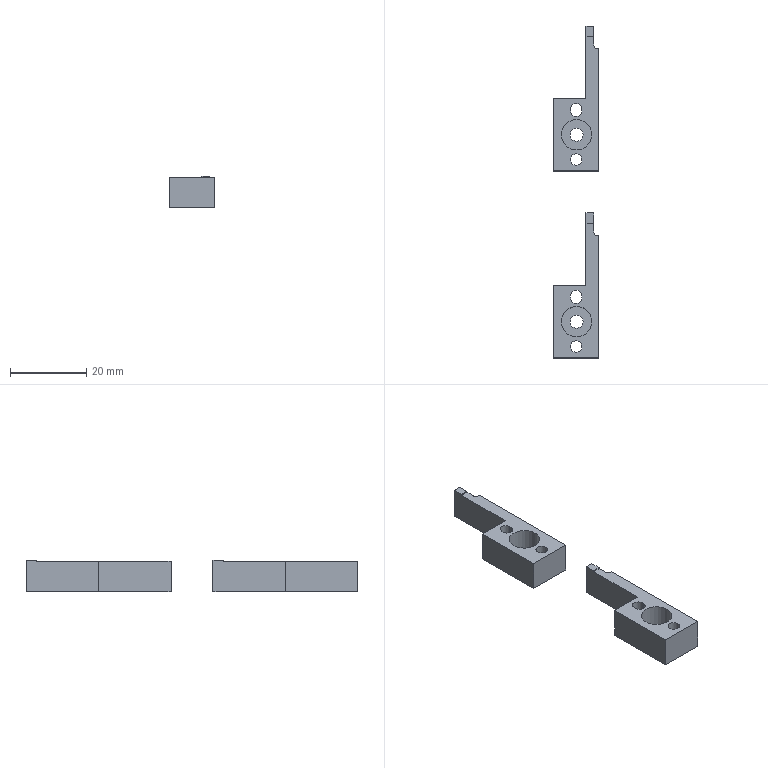Part | 2 solids | 42 faces | box 11.9 x 87 x 8.25 mm | volume 3631 mm3 | plane 30 | cylinder 12 | commonest cylinder face diameters 3 x6 2 x2 3.4 x2 8 x2
STEP:
#1=CARTESIAN_POINT('',(2.59,68.,8.25));
#2=VERTEX_POINT('',#1);
#3=CARTESIAN_POINT('',(2.59,65.3,8.25));
#4=VERTEX_POINT('',#3);
#5=CARTESIAN_POINT('',(2.59,68.,8.25));
#6=DIRECTION('',(0.,-1.,0.));
#7=VECTOR('',#6,1000.);
#8=LINE('',#5,#7);
#9=EDGE_CURVE('',#2,#4,#8,.T.);
#10=ORIENTED_EDGE('',*,*,#9,.T.);
#11=CARTESIAN_POINT('',(4.65,65.3,8.25));
#12=VERTEX_POINT('',#11);
#13=CARTESIAN_POINT('',(2.59,65.3,8.25));
#14=DIRECTION('',(1.,0.,0.));
#15=VECTOR('',#14,1000.);
#16=LINE('',#13,#15);
#17=EDGE_CURVE('',#4,#12,#16,.T.);
#18=ORIENTED_EDGE('',*,*,#17,.T.);
#19=CARTESIAN_POINT('',(4.65,68.,8.25));
#20=VERTEX_POINT('',#19);
#21=CARTESIAN_POINT('',(4.65,68.,8.25));
#22=DIRECTION('',(0.,1.,0.));
#23=VECTOR('',#22,1000.);
#24=LINE('',#21,#23);
#25=EDGE_CURVE('',#12,#20,#24,.T.);
#26=ORIENTED_EDGE('',*,*,#25,.T.);
#27=CARTESIAN_POINT('',(2.59,68.,8.25));
#28=DIRECTION('',(-1.,0.,0.));
#29=VECTOR('',#28,1000.);
#30=LINE('',#27,#29);
#31=EDGE_CURVE('',#20,#2,#30,.T.);
#32=ORIENTED_EDGE('',*,*,#31,.T.);
#33=EDGE_LOOP('',(#10,#18,#26,#32));
#34=FACE_BOUND('',#33,.T.);
#35=CARTESIAN_POINT('',(0.,49.,8.25));
#36=DIRECTION('',(0.,0.,1.));
#37=DIRECTION('',(1.,0.,0.));
#38=AXIS2_PLACEMENT_3D('',#35,#36,#37);
#39=PLANE('',#38);
#40=ADVANCED_FACE('',(#34),#39,.T.);
#41=CARTESIAN_POINT('',(2.59,65.3,8.));
#42=VERTEX_POINT('',#41);
#43=CARTESIAN_POINT('',(4.65,65.3,8.));
#44=VERTEX_POINT('',#43);
#45=CARTESIAN_POINT('',(2.59,65.3,8.));
#46=DIRECTION('',(1.,0.,0.));
#47=VECTOR('',#46,1000.);
#48=LINE('',#45,#47);
#49=EDGE_CURVE('',#42,#44,#48,.T.);
#50=ORIENTED_EDGE('',*,*,#49,.T.);
#51=CARTESIAN_POINT('',(4.65,65.3,8.25));
#52=DIRECTION('',(0.,0.,-1.));
#53=VECTOR('',#52,1000.);
#54=LINE('',#51,#53);
#55=EDGE_CURVE('',#12,#44,#54,.T.);
#56=ORIENTED_EDGE('',*,*,#55,.F.);
#57=ORIENTED_EDGE('',*,*,#17,.F.);
#58=CARTESIAN_POINT('',(2.59,65.3,8.25));
#59=DIRECTION('',(0.,0.,-1.));
#60=VECTOR('',#59,1000.);
#61=LINE('',#58,#60);
#62=EDGE_CURVE('',#4,#42,#61,.T.);
#63=ORIENTED_EDGE('',*,*,#62,.T.);
#64=EDGE_LOOP('',(#50,#56,#57,#63));
#65=FACE_BOUND('',#64,.T.);
#66=CARTESIAN_POINT('',(2.59,65.3,8.25));
#67=DIRECTION('',(0.,1.,0.));
#68=DIRECTION('',(0.,0.,1.));
#69=AXIS2_PLACEMENT_3D('',#66,#67,#68);
#70=PLANE('',#69);
#71=ADVANCED_FACE('',(#65),#70,.F.);
#72=CARTESIAN_POINT('',(5.65,62.,8.));
#73=VERTEX_POINT('',#72);
#74=CARTESIAN_POINT('',(4.65,63.,8.));
#75=VERTEX_POINT('',#74);
#76=CARTESIAN_POINT('',(5.65,63.,8.));
#77=DIRECTION('',(0.,0.,-1.));
#78=DIRECTION('',(-1.,0.,0.));
#79=AXIS2_PLACEMENT_3D('',#76,#77,#78);
#80=CIRCLE('',#79,1.);
#81=EDGE_CURVE('',#73,#75,#80,.T.);
#82=ORIENTED_EDGE('',*,*,#81,.F.);
#83=CARTESIAN_POINT('',(5.65,62.,0.));
#84=VERTEX_POINT('',#83);
#85=CARTESIAN_POINT('',(5.65,62.,8.));
#86=DIRECTION('',(0.,0.,1.));
#87=VECTOR('',#86,1000.);
#88=LINE('',#85,#87);
#89=EDGE_CURVE('',#84,#73,#88,.T.);
#90=ORIENTED_EDGE('',*,*,#89,.F.);
#91=CARTESIAN_POINT('',(4.65,63.,0.));
#92=VERTEX_POINT('',#91);
#93=CARTESIAN_POINT('',(5.65,63.,0.));
#94=DIRECTION('',(0.,0.,1.));
#95=DIRECTION('',(-1.,0.,0.));
#96=AXIS2_PLACEMENT_3D('',#93,#94,#95);
#97=CIRCLE('',#96,1.);
#98=EDGE_CURVE('',#92,#84,#97,.T.);
#99=ORIENTED_EDGE('',*,*,#98,.F.);
#100=CARTESIAN_POINT('',(4.65,63.,0.));
#101=DIRECTION('',(0.,0.,-1.));
#102=VECTOR('',#101,1000.);
#103=LINE('',#100,#102);
#104=EDGE_CURVE('',#75,#92,#103,.T.);
#105=ORIENTED_EDGE('',*,*,#104,.F.);
#106=EDGE_LOOP('',(#82,#90,#99,#105));
#107=FACE_BOUND('',#106,.T.);
#108=CARTESIAN_POINT('',(5.65,63.,8.));
#109=DIRECTION('',(0.,0.,1.));
#110=DIRECTION('',(1.,0.,0.));
#111=AXIS2_PLACEMENT_3D('',#108,#109,#110);
#112=CYLINDRICAL_SURFACE('',#111,1.);
#113=ADVANCED_FACE('',(#107),#112,.F.);
#114=CARTESIAN_POINT('',(5.95,62.,0.));
#115=VERTEX_POINT('',#114);
#116=CARTESIAN_POINT('',(5.95,62.,0.));
#117=DIRECTION('',(-1.,0.,0.));
#118=VECTOR('',#117,1000.);
#119=LINE('',#116,#118);
#120=EDGE_CURVE('',#115,#84,#119,.T.);
#121=ORIENTED_EDGE('',*,*,#120,.T.);
#122=ORIENTED_EDGE('',*,*,#89,.T.);
#123=CARTESIAN_POINT('',(5.95,62.,8.));
#124=VERTEX_POINT('',#123);
#125=CARTESIAN_POINT('',(5.95,62.,8.));
#126=DIRECTION('',(-1.,0.,0.));
#127=VECTOR('',#126,1000.);
#128=LINE('',#125,#127);
#129=EDGE_CURVE('',#124,#73,#128,.T.);
#130=ORIENTED_EDGE('',*,*,#129,.F.);
#131=CARTESIAN_POINT('',(5.95,62.,8.));
#132=DIRECTION('',(0.,0.,-1.));
#133=VECTOR('',#132,1000.);
#134=LINE('',#131,#133);
#135=EDGE_CURVE('',#124,#115,#134,.T.);
#136=ORIENTED_EDGE('',*,*,#135,.T.);
#137=EDGE_LOOP('',(#121,#122,#130,#136));
#138=FACE_BOUND('',#137,.T.);
#139=CARTESIAN_POINT('',(5.95,62.,8.));
#140=DIRECTION('',(0.,-1.,0.));
#141=DIRECTION('',(0.,0.,-1.));
#142=AXIS2_PLACEMENT_3D('',#139,#140,#141);
#143=PLANE('',#142);
#144=ADVANCED_FACE('',(#138),#143,.F.);
#145=CARTESIAN_POINT('',(4.65,68.,8.));
#146=DIRECTION('',(0.,1.,0.));
#147=VECTOR('',#146,1000.);
#148=LINE('',#145,#147);
#149=EDGE_CURVE('',#75,#44,#148,.T.);
#150=ORIENTED_EDGE('',*,*,#149,.F.);
#151=ORIENTED_EDGE('',*,*,#104,.T.);
#152=CARTESIAN_POINT('',(4.65,68.,0.));
#153=VERTEX_POINT('',#152);
#154=CARTESIAN_POINT('',(4.65,68.,0.));
#155=DIRECTION('',(0.,1.,0.));
#156=VECTOR('',#155,1000.);
#157=LINE('',#154,#156);
#158=EDGE_CURVE('',#92,#153,#157,.T.);
#159=ORIENTED_EDGE('',*,*,#158,.T.);
#160=CARTESIAN_POINT('',(4.65,68.,8.));
#161=DIRECTION('',(0.,0.,-1.));
#162=VECTOR('',#161,1000.);
#163=LINE('',#160,#162);
#164=EDGE_CURVE('',#20,#153,#163,.T.);
#165=ORIENTED_EDGE('',*,*,#164,.F.);
#166=ORIENTED_EDGE('',*,*,#25,.F.);
#167=ORIENTED_EDGE('',*,*,#55,.T.);
#168=EDGE_LOOP('',(#150,#151,#159,#165,#166,#167));
#169=FACE_BOUND('',#168,.T.);
#170=CARTESIAN_POINT('',(4.65,68.,8.));
#171=DIRECTION('',(-1.,0.,0.));
#172=DIRECTION('',(0.,-1.,0.));
#173=AXIS2_PLACEMENT_3D('',#170,#171,#172);
#174=PLANE('',#173);
#175=ADVANCED_FACE('',(#169),#174,.F.);
#176=CARTESIAN_POINT('',(2.59,68.,0.));
#177=VERTEX_POINT('',#176);
#178=CARTESIAN_POINT('',(2.59,49.,0.));
#179=VERTEX_POINT('',#178);
#180=CARTESIAN_POINT('',(2.59,68.,0.));
#181=DIRECTION('',(0.,-1.,0.));
#182=VECTOR('',#181,1000.);
#183=LINE('',#180,#182);
#184=EDGE_CURVE('',#177,#179,#183,.T.);
#185=ORIENTED_EDGE('',*,*,#184,.T.);
#186=CARTESIAN_POINT('',(2.59,49.,8.));
#187=VERTEX_POINT('',#186);
#188=CARTESIAN_POINT('',(2.59,49.,8.));
#189=DIRECTION('',(0.,0.,-1.));
#190=VECTOR('',#189,1000.);
#191=LINE('',#188,#190);
#192=EDGE_CURVE('',#187,#179,#191,.T.);
#193=ORIENTED_EDGE('',*,*,#192,.F.);
#194=CARTESIAN_POINT('',(2.59,68.,8.));
#195=DIRECTION('',(0.,-1.,0.));
#196=VECTOR('',#195,1000.);
#197=LINE('',#194,#196);
#198=EDGE_CURVE('',#42,#187,#197,.T.);
#199=ORIENTED_EDGE('',*,*,#198,.F.);
#200=ORIENTED_EDGE('',*,*,#62,.F.);
#201=ORIENTED_EDGE('',*,*,#9,.F.);
#202=CARTESIAN_POINT('',(2.59,68.,8.));
#203=DIRECTION('',(0.,0.,-1.));
#204=VECTOR('',#203,1000.);
#205=LINE('',#202,#204);
#206=EDGE_CURVE('',#2,#177,#205,.T.);
#207=ORIENTED_EDGE('',*,*,#206,.T.);
#208=EDGE_LOOP('',(#185,#193,#199,#200,#201,#207));
#209=FACE_BOUND('',#208,.T.);
#210=CARTESIAN_POINT('',(2.59,68.,8.));
#211=DIRECTION('',(1.,0.,0.));
#212=DIRECTION('',(0.,1.,0.));
#213=AXIS2_PLACEMENT_3D('',#210,#211,#212);
#214=PLANE('',#213);
#215=ADVANCED_FACE('',(#209),#214,.F.);
#216=CARTESIAN_POINT('',(-5.95,49.,0.));
#217=VERTEX_POINT('',#216);
#218=CARTESIAN_POINT('',(-5.95,49.,0.));
#219=DIRECTION('',(-1.,0.,0.));
#220=VECTOR('',#219,1000.);
#221=LINE('',#218,#220);
#222=EDGE_CURVE('',#179,#217,#221,.T.);
#223=ORIENTED_EDGE('',*,*,#222,.T.);
#224=CARTESIAN_POINT('',(-5.95,49.,8.));
#225=VERTEX_POINT('',#224);
#226=CARTESIAN_POINT('',(-5.95,49.,8.));
#227=DIRECTION('',(0.,0.,-1.));
#228=VECTOR('',#227,1000.);
#229=LINE('',#226,#228);
#230=EDGE_CURVE('',#225,#217,#229,.T.);
#231=ORIENTED_EDGE('',*,*,#230,.F.);
#232=CARTESIAN_POINT('',(-5.95,49.,8.));
#233=DIRECTION('',(-1.,0.,0.));
#234=VECTOR('',#233,1000.);
#235=LINE('',#232,#234);
#236=EDGE_CURVE('',#187,#225,#235,.T.);
#237=ORIENTED_EDGE('',*,*,#236,.F.);
#238=ORIENTED_EDGE('',*,*,#192,.T.);
#239=EDGE_LOOP('',(#223,#231,#237,#238));
#240=FACE_BOUND('',#239,.T.);
#241=CARTESIAN_POINT('',(-5.95,49.,8.));
#242=DIRECTION('',(0.,-1.,0.));
#243=DIRECTION('',(0.,0.,-1.));
#244=AXIS2_PLACEMENT_3D('',#241,#242,#243);
#245=PLANE('',#244);
#246=ADVANCED_FACE('',(#240),#245,.F.);
#247=CARTESIAN_POINT('',(4.15,39.5,2.));
#248=VERTEX_POINT('',#247);
#249=CARTESIAN_POINT('',(0.15,39.5,2.));
#250=DIRECTION('',(0.,0.,1.));
#251=DIRECTION('',(1.,0.,0.));
#252=AXIS2_PLACEMENT_3D('',#249,#250,#251);
#253=CIRCLE('',#252,4.);
#254=EDGE_CURVE('',#248,#248,#253,.T.);
#255=ORIENTED_EDGE('',*,*,#254,.T.);
#256=EDGE_LOOP('',(#255));
#257=FACE_BOUND('',#256,.T.);
#258=CARTESIAN_POINT('',(-1.55,39.5,2.));
#259=VERTEX_POINT('',#258);
#260=CARTESIAN_POINT('',(0.15,39.5,2.));
#261=DIRECTION('',(0.,0.,-1.));
#262=DIRECTION('',(-1.,0.,0.));
#263=AXIS2_PLACEMENT_3D('',#260,#261,#262);
#264=CIRCLE('',#263,1.7);
#265=EDGE_CURVE('',#259,#259,#264,.T.);
#266=ORIENTED_EDGE('',*,*,#265,.T.);
#267=EDGE_LOOP('',(#266));
#268=FACE_BOUND('',#267,.T.);
#269=CARTESIAN_POINT('',(0.15,39.5,2.));
#270=DIRECTION('',(0.,0.,-1.));
#271=DIRECTION('',(-1.,0.,0.));
#272=AXIS2_PLACEMENT_3D('',#269,#270,#271);
#273=PLANE('',#272);
#274=ADVANCED_FACE('',(#257,#268),#273,.F.);
#275=CARTESIAN_POINT('',(-1.45,46.25,0.));
#276=VERTEX_POINT('',#275);
#277=CARTESIAN_POINT('',(1.55,46.25,0.));
#278=VERTEX_POINT('',#277);
#279=CARTESIAN_POINT('',(0.05,46.25,0.));
#280=DIRECTION('',(0.,0.,-1.));
#281=DIRECTION('',(-1.,0.,0.));
#282=AXIS2_PLACEMENT_3D('',#279,#280,#281);
#283=CIRCLE('',#282,1.5);
#284=EDGE_CURVE('',#276,#278,#283,.T.);
#285=ORIENTED_EDGE('',*,*,#284,.T.);
#286=CARTESIAN_POINT('',(1.55,46.25,8.));
#287=VERTEX_POINT('',#286);
#288=CARTESIAN_POINT('',(1.55,46.25,8.));
#289=DIRECTION('',(0.,0.,1.));
#290=VECTOR('',#289,1000.);
#291=LINE('',#288,#290);
#292=EDGE_CURVE('',#278,#287,#291,.T.);
#293=ORIENTED_EDGE('',*,*,#292,.T.);
#294=CARTESIAN_POINT('',(-1.45,46.25,8.));
#295=VERTEX_POINT('',#294);
#296=CARTESIAN_POINT('',(0.05,46.25,8.));
#297=DIRECTION('',(0.,0.,-1.));
#298=DIRECTION('',(-1.,0.,0.));
#299=AXIS2_PLACEMENT_3D('',#296,#297,#298);
#300=CIRCLE('',#299,1.5);
#301=EDGE_CURVE('',#295,#287,#300,.T.);
#302=ORIENTED_EDGE('',*,*,#301,.F.);
#303=CARTESIAN_POINT('',(-1.45,46.25,0.));
#304=DIRECTION('',(0.,0.,1.));
#305=VECTOR('',#304,1000.);
#306=LINE('',#303,#305);
#307=EDGE_CURVE('',#276,#295,#306,.T.);
#308=ORIENTED_EDGE('',*,*,#307,.F.);
#309=EDGE_LOOP('',(#285,#293,#302,#308));
#310=FACE_BOUND('',#309,.T.);
#311=CARTESIAN_POINT('',(0.05,46.25,0.));
#312=DIRECTION('',(0.,0.,-1.));
#313=DIRECTION('',(-1.,0.,0.));
#314=AXIS2_PLACEMENT_3D('',#311,#312,#313);
#315=CYLINDRICAL_SURFACE('',#314,1.5);
#316=ADVANCED_FACE('',(#310),#315,.F.);
#317=CARTESIAN_POINT('',(1.55,45.75,8.));
#318=VERTEX_POINT('',#317);
#319=CARTESIAN_POINT('',(-1.45,45.75,8.));
#320=VERTEX_POINT('',#319);
#321=CARTESIAN_POINT('',(0.05,45.75,8.));
#322=DIRECTION('',(0.,0.,-1.));
#323=DIRECTION('',(-1.,0.,0.));
#324=AXIS2_PLACEMENT_3D('',#321,#322,#323);
#325=CIRCLE('',#324,1.5);
#326=EDGE_CURVE('',#318,#320,#325,.T.);
#327=ORIENTED_EDGE('',*,*,#326,.F.);
#328=CARTESIAN_POINT('',(1.55,45.75,0.));
#329=VERTEX_POINT('',#328);
#330=CARTESIAN_POINT('',(1.55,45.75,8.));
#331=DIRECTION('',(0.,0.,1.));
#332=VECTOR('',#331,1000.);
#333=LINE('',#330,#332);
#334=EDGE_CURVE('',#329,#318,#333,.T.);
#335=ORIENTED_EDGE('',*,*,#334,.F.);
#336=CARTESIAN_POINT('',(-1.45,45.75,0.));
#337=VERTEX_POINT('',#336);
#338=CARTESIAN_POINT('',(0.05,45.75,0.));
#339=DIRECTION('',(0.,0.,-1.));
#340=DIRECTION('',(-1.,0.,0.));
#341=AXIS2_PLACEMENT_3D('',#338,#339,#340);
#342=CIRCLE('',#341,1.5);
#343=EDGE_CURVE('',#329,#337,#342,.T.);
#344=ORIENTED_EDGE('',*,*,#343,.T.);
#345=CARTESIAN_POINT('',(-1.45,45.75,0.));
#346=DIRECTION('',(0.,0.,-1.));
#347=VECTOR('',#346,1000.);
#348=LINE('',#345,#347);
#349=EDGE_CURVE('',#320,#337,#348,.T.);
#350=ORIENTED_EDGE('',*,*,#349,.F.);
#351=EDGE_LOOP('',(#327,#335,#344,#350));
#352=FACE_BOUND('',#351,.T.);
#353=CARTESIAN_POINT('',(0.05,45.75,0.));
#354=DIRECTION('',(0.,0.,-1.));
#355=DIRECTION('',(-1.,0.,0.));
#356=AXIS2_PLACEMENT_3D('',#353,#354,#355);
#357=CYLINDRICAL_SURFACE('',#356,1.5);
#358=ADVANCED_FACE('',(#352),#357,.F.);
#359=CARTESIAN_POINT('',(-1.45,46.25,0.));
#360=DIRECTION('',(0.,-1.,0.));
#361=VECTOR('',#360,1000.);
#362=LINE('',#359,#361);
#363=EDGE_CURVE('',#276,#337,#362,.T.);
#364=ORIENTED_EDGE('',*,*,#363,.F.);
#365=ORIENTED_EDGE('',*,*,#307,.T.);
#366=CARTESIAN_POINT('',(-1.45,46.25,8.));
#367=DIRECTION('',(0.,-1.,0.));
#368=VECTOR('',#367,1000.);
#369=LINE('',#366,#368);
#370=EDGE_CURVE('',#295,#320,#369,.T.);
#371=ORIENTED_EDGE('',*,*,#370,.T.);
#372=ORIENTED_EDGE('',*,*,#349,.T.);
#373=EDGE_LOOP('',(#364,#365,#371,#372));
#374=FACE_BOUND('',#373,.T.);
#375=CARTESIAN_POINT('',(-1.45,46.25,0.));
#376=DIRECTION('',(-1.,0.,0.));
#377=DIRECTION('',(0.,-1.,0.));
#378=AXIS2_PLACEMENT_3D('',#375,#376,#377);
#379=PLANE('',#378);
#380=ADVANCED_FACE('',(#374),#379,.F.);
#381=CARTESIAN_POINT('',(1.55,46.25,0.));
#382=DIRECTION('',(0.,-1.,0.));
#383=VECTOR('',#382,1000.);
#384=LINE('',#381,#383);
#385=EDGE_CURVE('',#278,#329,#384,.T.);
#386=ORIENTED_EDGE('',*,*,#385,.T.);
#387=ORIENTED_EDGE('',*,*,#334,.T.);
#388=CARTESIAN_POINT('',(1.55,46.25,8.));
#389=DIRECTION('',(0.,-1.,0.));
#390=VECTOR('',#389,1000.);
#391=LINE('',#388,#390);
#392=EDGE_CURVE('',#287,#318,#391,.T.);
#393=ORIENTED_EDGE('',*,*,#392,.F.);
#394=ORIENTED_EDGE('',*,*,#292,.F.);
#395=EDGE_LOOP('',(#386,#387,#393,#394));
#396=FACE_BOUND('',#395,.T.);
#397=CARTESIAN_POINT('',(1.55,46.25,8.));
#398=DIRECTION('',(1.,0.,0.));
#399=DIRECTION('',(0.,1.,0.));
#400=AXIS2_PLACEMENT_3D('',#397,#398,#399);
#401=PLANE('',#400);
#402=ADVANCED_FACE('',(#396),#401,.F.);
#403=CARTESIAN_POINT('',(-5.95,30.,0.));
#404=VERTEX_POINT('',#403);
#405=CARTESIAN_POINT('',(5.95,30.,0.));
#406=VERTEX_POINT('',#405);
#407=CARTESIAN_POINT('',(-5.95,30.,0.));
#408=DIRECTION('',(1.,0.,0.));
#409=VECTOR('',#408,1000.);
#410=LINE('',#407,#409);
#411=EDGE_CURVE('',#404,#406,#410,.T.);
#412=ORIENTED_EDGE('',*,*,#411,.T.);
#413=CARTESIAN_POINT('',(5.95,30.,8.));
#414=VERTEX_POINT('',#413);
#415=CARTESIAN_POINT('',(5.95,30.,8.));
#416=DIRECTION('',(0.,0.,-1.));
#417=VECTOR('',#416,1000.);
#418=LINE('',#415,#417);
#419=EDGE_CURVE('',#414,#406,#418,.T.);
#420=ORIENTED_EDGE('',*,*,#419,.F.);
#421=CARTESIAN_POINT('',(-5.95,30.,8.));
#422=VERTEX_POINT('',#421);
#423=CARTESIAN_POINT('',(-5.95,30.,8.));
#424=DIRECTION('',(1.,0.,0.));
#425=VECTOR('',#424,1000.);
#426=LINE('',#423,#425);
#427=EDGE_CURVE('',#422,#414,#426,.T.);
#428=ORIENTED_EDGE('',*,*,#427,.F.);
#429=CARTESIAN_POINT('',(-5.95,30.,8.));
#430=DIRECTION('',(0.,0.,-1.));
#431=VECTOR('',#430,1000.);
#432=LINE('',#429,#431);
#433=EDGE_CURVE('',#422,#404,#432,.T.);
#434=ORIENTED_EDGE('',*,*,#433,.T.);
#435=EDGE_LOOP('',(#412,#420,#428,#434));
#436=FACE_BOUND('',#435,.T.);
#437=CARTESIAN_POINT('',(-5.95,30.,8.));
#438=DIRECTION('',(0.,1.,0.));
#439=DIRECTION('',(0.,0.,1.));
#440=AXIS2_PLACEMENT_3D('',#437,#438,#439);
#441=PLANE('',#440);
#442=ADVANCED_FACE('',(#436),#441,.F.);
#443=CARTESIAN_POINT('',(-5.95,30.,8.));
#444=DIRECTION('',(0.,-1.,0.));
#445=VECTOR('',#444,1000.);
#446=LINE('',#443,#445);
#447=EDGE_CURVE('',#225,#422,#446,.T.);
#448=ORIENTED_EDGE('',*,*,#447,.F.);
#449=ORIENTED_EDGE('',*,*,#230,.T.);
#450=CARTESIAN_POINT('',(-5.95,30.,0.));
#451=DIRECTION('',(0.,-1.,0.));
#452=VECTOR('',#451,1000.);
#453=LINE('',#450,#452);
#454=EDGE_CURVE('',#217,#404,#453,.T.);
#455=ORIENTED_EDGE('',*,*,#454,.T.);
#456=ORIENTED_EDGE('',*,*,#433,.F.);
#457=EDGE_LOOP('',(#448,#449,#455,#456));
#458=FACE_BOUND('',#457,.T.);
#459=CARTESIAN_POINT('',(-5.95,30.,8.));
#460=DIRECTION('',(1.,0.,0.));
#461=DIRECTION('',(0.,0.,-1.));
#462=AXIS2_PLACEMENT_3D('',#459,#460,#461);
#463=PLANE('',#462);
#464=ADVANCED_FACE('',(#458),#463,.F.);
#465=ORIENTED_EDGE('',*,*,#206,.F.);
#466=ORIENTED_EDGE('',*,*,#31,.F.);
#467=ORIENTED_EDGE('',*,*,#164,.T.);
#468=CARTESIAN_POINT('',(-5.95,68.,0.));
#469=DIRECTION('',(-1.,0.,0.));
#470=VECTOR('',#469,1000.);
#471=LINE('',#468,#470);
#472=EDGE_CURVE('',#153,#177,#471,.T.);
#473=ORIENTED_EDGE('',*,*,#472,.T.);
#474=EDGE_LOOP('',(#465,#466,#467,#473));
#475=FACE_BOUND('',#474,.T.);
#476=CARTESIAN_POINT('',(-5.95,68.,8.));
#477=DIRECTION('',(0.,-1.,0.));
#478=DIRECTION('',(0.,0.,-1.));
#479=AXIS2_PLACEMENT_3D('',#476,#477,#478);
#480=PLANE('',#479);
#481=ADVANCED_FACE('',(#475),#480,.F.);
#482=CARTESIAN_POINT('',(5.95,30.,0.));
#483=DIRECTION('',(0.,1.,0.));
#484=VECTOR('',#483,1000.);
#485=LINE('',#482,#484);
#486=EDGE_CURVE('',#406,#115,#485,.T.);
#487=ORIENTED_EDGE('',*,*,#486,.T.);
#488=ORIENTED_EDGE('',*,*,#135,.F.);
#489=CARTESIAN_POINT('',(5.95,30.,8.));
#490=DIRECTION('',(0.,1.,0.));
#491=VECTOR('',#490,1000.);
#492=LINE('',#489,#491);
#493=EDGE_CURVE('',#414,#124,#492,.T.);
#494=ORIENTED_EDGE('',*,*,#493,.F.);
#495=ORIENTED_EDGE('',*,*,#419,.T.);
#496=EDGE_LOOP('',(#487,#488,#494,#495));
#497=FACE_BOUND('',#496,.T.);
#498=CARTESIAN_POINT('',(5.95,30.,8.));
#499=DIRECTION('',(-1.,0.,0.));
#500=DIRECTION('',(0.,0.,1.));
#501=AXIS2_PLACEMENT_3D('',#498,#499,#500);
#502=PLANE('',#501);
#503=ADVANCED_FACE('',(#497),#502,.F.);
#504=ORIENTED_EDGE('',*,*,#363,.T.);
#505=ORIENTED_EDGE('',*,*,#343,.F.);
#506=ORIENTED_EDGE('',*,*,#385,.F.);
#507=ORIENTED_EDGE('',*,*,#284,.F.);
#508=EDGE_LOOP('',(#504,#505,#506,#507));
#509=FACE_BOUND('',#508,.T.);
#510=CARTESIAN_POINT('',(-1.45,33.,0.));
#511=VERTEX_POINT('',#510);
#512=CARTESIAN_POINT('',(0.05,33.,0.));
#513=DIRECTION('',(0.,0.,-1.));
#514=DIRECTION('',(-1.,0.,0.));
#515=AXIS2_PLACEMENT_3D('',#512,#513,#514);
#516=CIRCLE('',#515,1.5);
#517=EDGE_CURVE('',#511,#511,#516,.T.);
#518=ORIENTED_EDGE('',*,*,#517,.F.);
#519=EDGE_LOOP('',(#518));
#520=FACE_BOUND('',#519,.T.);
#521=CARTESIAN_POINT('',(1.85,39.5,0.));
#522=VERTEX_POINT('',#521);
#523=CARTESIAN_POINT('',(0.15,39.5,0.));
#524=DIRECTION('',(0.,0.,1.));
#525=DIRECTION('',(1.,0.,0.));
#526=AXIS2_PLACEMENT_3D('',#523,#524,#525);
#527=CIRCLE('',#526,1.7);
#528=EDGE_CURVE('',#522,#522,#527,.T.);
#529=ORIENTED_EDGE('',*,*,#528,.T.);
#530=EDGE_LOOP('',(#529));
#531=FACE_BOUND('',#530,.T.);
#532=ORIENTED_EDGE('',*,*,#158,.F.);
#533=ORIENTED_EDGE('',*,*,#98,.T.);
#534=ORIENTED_EDGE('',*,*,#120,.F.);
#535=ORIENTED_EDGE('',*,*,#486,.F.);
#536=ORIENTED_EDGE('',*,*,#411,.F.);
#537=ORIENTED_EDGE('',*,*,#454,.F.);
#538=ORIENTED_EDGE('',*,*,#222,.F.);
#539=ORIENTED_EDGE('',*,*,#184,.F.);
#540=ORIENTED_EDGE('',*,*,#472,.F.);
#541=EDGE_LOOP('',(#532,#533,#534,#535,#536,#537,#538,#539,#540));
#542=FACE_BOUND('',#541,.T.);
#543=CARTESIAN_POINT('',(0.,49.,0.));
#544=DIRECTION('',(0.,0.,-1.));
#545=DIRECTION('',(-1.,0.,0.));
#546=AXIS2_PLACEMENT_3D('',#543,#544,#545);
#547=PLANE('',#546);
#548=ADVANCED_FACE('',(#509,#520,#531,#542),#547,.T.);
#549=ORIENTED_EDGE('',*,*,#49,.F.);
#550=ORIENTED_EDGE('',*,*,#198,.T.);
#551=ORIENTED_EDGE('',*,*,#236,.T.);
#552=ORIENTED_EDGE('',*,*,#447,.T.);
#553=ORIENTED_EDGE('',*,*,#427,.T.);
#554=ORIENTED_EDGE('',*,*,#493,.T.);
#555=ORIENTED_EDGE('',*,*,#129,.T.);
#556=ORIENTED_EDGE('',*,*,#81,.T.);
#557=ORIENTED_EDGE('',*,*,#149,.T.);
#558=EDGE_LOOP('',(#549,#550,#551,#552,#553,#554,#555,#556,#557));
#559=FACE_BOUND('',#558,.T.);
#560=CARTESIAN_POINT('',(4.15,39.5,8.));
#561=VERTEX_POINT('',#560);
#562=CARTESIAN_POINT('',(0.15,39.5,8.));
#563=DIRECTION('',(0.,0.,1.));
#564=DIRECTION('',(1.,0.,0.));
#565=AXIS2_PLACEMENT_3D('',#562,#563,#564);
#566=CIRCLE('',#565,4.);
#567=EDGE_CURVE('',#561,#561,#566,.T.);
#568=ORIENTED_EDGE('',*,*,#567,.F.);
#569=EDGE_LOOP('',(#568));
#570=FACE_BOUND('',#569,.T.);
#571=CARTESIAN_POINT('',(-1.45,33.,8.));
#572=VERTEX_POINT('',#571);
#573=CARTESIAN_POINT('',(0.05,33.,8.));
#574=DIRECTION('',(0.,0.,-1.));
#575=DIRECTION('',(-1.,0.,0.));
#576=AXIS2_PLACEMENT_3D('',#573,#574,#575);
#577=CIRCLE('',#576,1.5);
#578=EDGE_CURVE('',#572,#572,#577,.T.);
#579=ORIENTED_EDGE('',*,*,#578,.T.);
#580=EDGE_LOOP('',(#579));
#581=FACE_BOUND('',#580,.T.);
#582=ORIENTED_EDGE('',*,*,#392,.T.);
#583=ORIENTED_EDGE('',*,*,#326,.T.);
#584=ORIENTED_EDGE('',*,*,#370,.F.);
#585=ORIENTED_EDGE('',*,*,#301,.T.);
#586=EDGE_LOOP('',(#582,#583,#584,#585));
#587=FACE_BOUND('',#586,.T.);
#588=CARTESIAN_POINT('',(0.,49.,8.));
#589=DIRECTION('',(0.,0.,-1.));
#590=DIRECTION('',(-1.,0.,0.));
#591=AXIS2_PLACEMENT_3D('',#588,#589,#590);
#592=PLANE('',#591);
#593=ADVANCED_FACE('',(#559,#570,#581,#587),#592,.F.);
#594=ORIENTED_EDGE('',*,*,#517,.T.);
#595=EDGE_LOOP('',(#594));
#596=FACE_BOUND('',#595,.T.);
#597=ORIENTED_EDGE('',*,*,#578,.F.);
#598=EDGE_LOOP('',(#597));
#599=FACE_BOUND('',#598,.T.);
#600=CARTESIAN_POINT('',(0.05,33.,0.));
#601=DIRECTION('',(0.,0.,-1.));
#602=DIRECTION('',(-1.,0.,0.));
#603=AXIS2_PLACEMENT_3D('',#600,#601,#602);
#604=CYLINDRICAL_SURFACE('',#603,1.5);
#605=ADVANCED_FACE('',(#596,#599),#604,.F.);
#606=ORIENTED_EDGE('',*,*,#254,.F.);
#607=EDGE_LOOP('',(#606));
#608=FACE_BOUND('',#607,.T.);
#609=ORIENTED_EDGE('',*,*,#567,.T.);
#610=EDGE_LOOP('',(#609));
#611=FACE_BOUND('',#610,.T.);
#612=CARTESIAN_POINT('',(0.15,39.5,8.));
#613=DIRECTION('',(0.,0.,1.));
#614=DIRECTION('',(1.,0.,0.));
#615=AXIS2_PLACEMENT_3D('',#612,#613,#614);
#616=CYLINDRICAL_SURFACE('',#615,4.);
#617=ADVANCED_FACE('',(#608,#611),#616,.F.);
#618=ORIENTED_EDGE('',*,*,#528,.F.);
#619=EDGE_LOOP('',(#618));
#620=FACE_BOUND('',#619,.T.);
#621=ORIENTED_EDGE('',*,*,#265,.F.);
#622=EDGE_LOOP('',(#621));
#623=FACE_BOUND('',#622,.T.);
#624=CARTESIAN_POINT('',(0.15,39.5,8.));
#625=DIRECTION('',(0.,0.,1.));
#626=DIRECTION('',(1.,0.,0.));
#627=AXIS2_PLACEMENT_3D('',#624,#625,#626);
#628=CYLINDRICAL_SURFACE('',#627,1.7);
#629=ADVANCED_FACE('',(#620,#623),#628,.F.);
#630=CLOSED_SHELL('',(#40,#71,#113,#144,#175,#215,#246,#274,#316,#358,#380,#402,#442,#464,#481,#503,#548,#593,#605,#617,#629));
#631=MANIFOLD_SOLID_BREP('',#630);
#632=CARTESIAN_POINT('',(2.59,19.,8.25));
#633=VERTEX_POINT('',#632);
#634=CARTESIAN_POINT('',(2.59,16.3,8.25));
#635=VERTEX_POINT('',#634);
#636=CARTESIAN_POINT('',(2.59,19.,8.25));
#637=DIRECTION('',(0.,-1.,0.));
#638=VECTOR('',#637,1000.);
#639=LINE('',#636,#638);
#640=EDGE_CURVE('',#633,#635,#639,.T.);
#641=ORIENTED_EDGE('',*,*,#640,.T.);
#642=CARTESIAN_POINT('',(4.65,16.3,8.25));
#643=VERTEX_POINT('',#642);
#644=CARTESIAN_POINT('',(2.59,16.3,8.25));
#645=DIRECTION('',(1.,0.,0.));
#646=VECTOR('',#645,1000.);
#647=LINE('',#644,#646);
#648=EDGE_CURVE('',#635,#643,#647,.T.);
#649=ORIENTED_EDGE('',*,*,#648,.T.);
#650=CARTESIAN_POINT('',(4.65,19.,8.25));
#651=VERTEX_POINT('',#650);
#652=CARTESIAN_POINT('',(4.65,19.,8.25));
#653=DIRECTION('',(0.,1.,0.));
#654=VECTOR('',#653,1000.);
#655=LINE('',#652,#654);
#656=EDGE_CURVE('',#643,#651,#655,.T.);
#657=ORIENTED_EDGE('',*,*,#656,.T.);
#658=CARTESIAN_POINT('',(2.59,19.,8.25));
#659=DIRECTION('',(-1.,0.,0.));
#660=VECTOR('',#659,1000.);
#661=LINE('',#658,#660);
#662=EDGE_CURVE('',#651,#633,#661,.T.);
#663=ORIENTED_EDGE('',*,*,#662,.T.);
#664=EDGE_LOOP('',(#641,#649,#657,#663));
#665=FACE_BOUND('',#664,.T.);
#666=CARTESIAN_POINT('',(0.,0.,8.25));
#667=DIRECTION('',(0.,0.,1.));
#668=DIRECTION('',(1.,0.,0.));
#669=AXIS2_PLACEMENT_3D('',#666,#667,#668);
#670=PLANE('',#669);
#671=ADVANCED_FACE('',(#665),#670,.T.);
#672=CARTESIAN_POINT('',(2.59,16.3,8.));
#673=VERTEX_POINT('',#672);
#674=CARTESIAN_POINT('',(4.65,16.3,8.));
#675=VERTEX_POINT('',#674);
#676=CARTESIAN_POINT('',(2.59,16.3,8.));
#677=DIRECTION('',(1.,0.,0.));
#678=VECTOR('',#677,1000.);
#679=LINE('',#676,#678);
#680=EDGE_CURVE('',#673,#675,#679,.T.);
#681=ORIENTED_EDGE('',*,*,#680,.T.);
#682=CARTESIAN_POINT('',(4.65,16.3,8.25));
#683=DIRECTION('',(0.,0.,-1.));
#684=VECTOR('',#683,1000.);
#685=LINE('',#682,#684);
#686=EDGE_CURVE('',#643,#675,#685,.T.);
#687=ORIENTED_EDGE('',*,*,#686,.F.);
#688=ORIENTED_EDGE('',*,*,#648,.F.);
#689=CARTESIAN_POINT('',(2.59,16.3,8.25));
#690=DIRECTION('',(0.,0.,-1.));
#691=VECTOR('',#690,1000.);
#692=LINE('',#689,#691);
#693=EDGE_CURVE('',#635,#673,#692,.T.);
#694=ORIENTED_EDGE('',*,*,#693,.T.);
#695=EDGE_LOOP('',(#681,#687,#688,#694));
#696=FACE_BOUND('',#695,.T.);
#697=CARTESIAN_POINT('',(2.59,16.3,8.25));
#698=DIRECTION('',(0.,1.,0.));
#699=DIRECTION('',(0.,0.,1.));
#700=AXIS2_PLACEMENT_3D('',#697,#698,#699);
#701=PLANE('',#700);
#702=ADVANCED_FACE('',(#696),#701,.F.);
#703=CARTESIAN_POINT('',(5.65,13.,8.));
#704=VERTEX_POINT('',#703);
#705=CARTESIAN_POINT('',(4.65,14.,8.));
#706=VERTEX_POINT('',#705);
#707=CARTESIAN_POINT('',(5.65,14.,8.));
#708=DIRECTION('',(0.,0.,-1.));
#709=DIRECTION('',(-1.,0.,0.));
#710=AXIS2_PLACEMENT_3D('',#707,#708,#709);
#711=CIRCLE('',#710,1.);
#712=EDGE_CURVE('',#704,#706,#711,.T.);
#713=ORIENTED_EDGE('',*,*,#712,.F.);
#714=CARTESIAN_POINT('',(5.65,13.,0.));
#715=VERTEX_POINT('',#714);
#716=CARTESIAN_POINT('',(5.65,13.,8.));
#717=DIRECTION('',(0.,0.,1.));
#718=VECTOR('',#717,1000.);
#719=LINE('',#716,#718);
#720=EDGE_CURVE('',#715,#704,#719,.T.);
#721=ORIENTED_EDGE('',*,*,#720,.F.);
#722=CARTESIAN_POINT('',(4.65,14.,0.));
#723=VERTEX_POINT('',#722);
#724=CARTESIAN_POINT('',(5.65,14.,0.));
#725=DIRECTION('',(0.,0.,1.));
#726=DIRECTION('',(-1.,0.,0.));
#727=AXIS2_PLACEMENT_3D('',#724,#725,#726);
#728=CIRCLE('',#727,1.);
#729=EDGE_CURVE('',#723,#715,#728,.T.);
#730=ORIENTED_EDGE('',*,*,#729,.F.);
#731=CARTESIAN_POINT('',(4.65,14.,0.));
#732=DIRECTION('',(0.,0.,-1.));
#733=VECTOR('',#732,1000.);
#734=LINE('',#731,#733);
#735=EDGE_CURVE('',#706,#723,#734,.T.);
#736=ORIENTED_EDGE('',*,*,#735,.F.);
#737=EDGE_LOOP('',(#713,#721,#730,#736));
#738=FACE_BOUND('',#737,.T.);
#739=CARTESIAN_POINT('',(5.65,14.,8.));
#740=DIRECTION('',(0.,0.,1.));
#741=DIRECTION('',(1.,0.,0.));
#742=AXIS2_PLACEMENT_3D('',#739,#740,#741);
#743=CYLINDRICAL_SURFACE('',#742,1.);
#744=ADVANCED_FACE('',(#738),#743,.F.);
#745=CARTESIAN_POINT('',(5.95,13.,0.));
#746=VERTEX_POINT('',#745);
#747=CARTESIAN_POINT('',(5.95,13.,0.));
#748=DIRECTION('',(-1.,0.,0.));
#749=VECTOR('',#748,1000.);
#750=LINE('',#747,#749);
#751=EDGE_CURVE('',#746,#715,#750,.T.);
#752=ORIENTED_EDGE('',*,*,#751,.T.);
#753=ORIENTED_EDGE('',*,*,#720,.T.);
#754=CARTESIAN_POINT('',(5.95,13.,8.));
#755=VERTEX_POINT('',#754);
#756=CARTESIAN_POINT('',(5.95,13.,8.));
#757=DIRECTION('',(-1.,0.,0.));
#758=VECTOR('',#757,1000.);
#759=LINE('',#756,#758);
#760=EDGE_CURVE('',#755,#704,#759,.T.);
#761=ORIENTED_EDGE('',*,*,#760,.F.);
#762=CARTESIAN_POINT('',(5.95,13.,8.));
#763=DIRECTION('',(0.,0.,-1.));
#764=VECTOR('',#763,1000.);
#765=LINE('',#762,#764);
#766=EDGE_CURVE('',#755,#746,#765,.T.);
#767=ORIENTED_EDGE('',*,*,#766,.T.);
#768=EDGE_LOOP('',(#752,#753,#761,#767));
#769=FACE_BOUND('',#768,.T.);
#770=CARTESIAN_POINT('',(5.95,13.,8.));
#771=DIRECTION('',(0.,-1.,0.));
#772=DIRECTION('',(0.,0.,-1.));
#773=AXIS2_PLACEMENT_3D('',#770,#771,#772);
#774=PLANE('',#773);
#775=ADVANCED_FACE('',(#769),#774,.F.);
#776=CARTESIAN_POINT('',(4.65,19.,8.));
#777=DIRECTION('',(0.,1.,0.));
#778=VECTOR('',#777,1000.);
#779=LINE('',#776,#778);
#780=EDGE_CURVE('',#706,#675,#779,.T.);
#781=ORIENTED_EDGE('',*,*,#780,.F.);
#782=ORIENTED_EDGE('',*,*,#735,.T.);
#783=CARTESIAN_POINT('',(4.65,19.,0.));
#784=VERTEX_POINT('',#783);
#785=CARTESIAN_POINT('',(4.65,19.,0.));
#786=DIRECTION('',(0.,1.,0.));
#787=VECTOR('',#786,1000.);
#788=LINE('',#785,#787);
#789=EDGE_CURVE('',#723,#784,#788,.T.);
#790=ORIENTED_EDGE('',*,*,#789,.T.);
#791=CARTESIAN_POINT('',(4.65,19.,8.));
#792=DIRECTION('',(0.,0.,-1.));
#793=VECTOR('',#792,1000.);
#794=LINE('',#791,#793);
#795=EDGE_CURVE('',#651,#784,#794,.T.);
#796=ORIENTED_EDGE('',*,*,#795,.F.);
#797=ORIENTED_EDGE('',*,*,#656,.F.);
#798=ORIENTED_EDGE('',*,*,#686,.T.);
#799=EDGE_LOOP('',(#781,#782,#790,#796,#797,#798));
#800=FACE_BOUND('',#799,.T.);
#801=CARTESIAN_POINT('',(4.65,19.,8.));
#802=DIRECTION('',(-1.,0.,0.));
#803=DIRECTION('',(0.,-1.,0.));
#804=AXIS2_PLACEMENT_3D('',#801,#802,#803);
#805=PLANE('',#804);
#806=ADVANCED_FACE('',(#800),#805,.F.);
#807=CARTESIAN_POINT('',(2.59,19.,0.));
#808=VERTEX_POINT('',#807);
#809=CARTESIAN_POINT('',(2.59,0.,0.));
#810=VERTEX_POINT('',#809);
#811=CARTESIAN_POINT('',(2.59,19.,0.));
#812=DIRECTION('',(0.,-1.,0.));
#813=VECTOR('',#812,1000.);
#814=LINE('',#811,#813);
#815=EDGE_CURVE('',#808,#810,#814,.T.);
#816=ORIENTED_EDGE('',*,*,#815,.T.);
#817=CARTESIAN_POINT('',(2.59,0.,8.));
#818=VERTEX_POINT('',#817);
#819=CARTESIAN_POINT('',(2.59,0.,8.));
#820=DIRECTION('',(0.,0.,-1.));
#821=VECTOR('',#820,1000.);
#822=LINE('',#819,#821);
#823=EDGE_CURVE('',#818,#810,#822,.T.);
#824=ORIENTED_EDGE('',*,*,#823,.F.);
#825=CARTESIAN_POINT('',(2.59,19.,8.));
#826=DIRECTION('',(0.,-1.,0.));
#827=VECTOR('',#826,1000.);
#828=LINE('',#825,#827);
#829=EDGE_CURVE('',#673,#818,#828,.T.);
#830=ORIENTED_EDGE('',*,*,#829,.F.);
#831=ORIENTED_EDGE('',*,*,#693,.F.);
#832=ORIENTED_EDGE('',*,*,#640,.F.);
#833=CARTESIAN_POINT('',(2.59,19.,8.));
#834=DIRECTION('',(0.,0.,-1.));
#835=VECTOR('',#834,1000.);
#836=LINE('',#833,#835);
#837=EDGE_CURVE('',#633,#808,#836,.T.);
#838=ORIENTED_EDGE('',*,*,#837,.T.);
#839=EDGE_LOOP('',(#816,#824,#830,#831,#832,#838));
#840=FACE_BOUND('',#839,.T.);
#841=CARTESIAN_POINT('',(2.59,19.,8.));
#842=DIRECTION('',(1.,0.,0.));
#843=DIRECTION('',(0.,1.,0.));
#844=AXIS2_PLACEMENT_3D('',#841,#842,#843);
#845=PLANE('',#844);
#846=ADVANCED_FACE('',(#840),#845,.F.);
#847=CARTESIAN_POINT('',(-5.95,0.,0.));
#848=VERTEX_POINT('',#847);
#849=CARTESIAN_POINT('',(-5.95,0.,0.));
#850=DIRECTION('',(-1.,0.,0.));
#851=VECTOR('',#850,1000.);
#852=LINE('',#849,#851);
#853=EDGE_CURVE('',#810,#848,#852,.T.);
#854=ORIENTED_EDGE('',*,*,#853,.T.);
#855=CARTESIAN_POINT('',(-5.95,0.,8.));
#856=VERTEX_POINT('',#855);
#857=CARTESIAN_POINT('',(-5.95,0.,8.));
#858=DIRECTION('',(0.,0.,-1.));
#859=VECTOR('',#858,1000.);
#860=LINE('',#857,#859);
#861=EDGE_CURVE('',#856,#848,#860,.T.);
#862=ORIENTED_EDGE('',*,*,#861,.F.);
#863=CARTESIAN_POINT('',(-5.95,0.,8.));
#864=DIRECTION('',(-1.,0.,0.));
#865=VECTOR('',#864,1000.);
#866=LINE('',#863,#865);
#867=EDGE_CURVE('',#818,#856,#866,.T.);
#868=ORIENTED_EDGE('',*,*,#867,.F.);
#869=ORIENTED_EDGE('',*,*,#823,.T.);
#870=EDGE_LOOP('',(#854,#862,#868,#869));
#871=FACE_BOUND('',#870,.T.);
#872=CARTESIAN_POINT('',(-5.95,0.,8.));
#873=DIRECTION('',(0.,-1.,0.));
#874=DIRECTION('',(0.,0.,-1.));
#875=AXIS2_PLACEMENT_3D('',#872,#873,#874);
#876=PLANE('',#875);
#877=ADVANCED_FACE('',(#871),#876,.F.);
#878=CARTESIAN_POINT('',(4.15,-9.5,2.));
#879=VERTEX_POINT('',#878);
#880=CARTESIAN_POINT('',(0.15,-9.5,2.));
#881=DIRECTION('',(0.,0.,1.));
#882=DIRECTION('',(1.,0.,0.));
#883=AXIS2_PLACEMENT_3D('',#880,#881,#882);
#884=CIRCLE('',#883,4.);
#885=EDGE_CURVE('',#879,#879,#884,.T.);
#886=ORIENTED_EDGE('',*,*,#885,.T.);
#887=EDGE_LOOP('',(#886));
#888=FACE_BOUND('',#887,.T.);
#889=CARTESIAN_POINT('',(-1.55,-9.5,2.));
#890=VERTEX_POINT('',#889);
#891=CARTESIAN_POINT('',(0.15,-9.5,2.));
#892=DIRECTION('',(0.,0.,-1.));
#893=DIRECTION('',(-1.,0.,0.));
#894=AXIS2_PLACEMENT_3D('',#891,#892,#893);
#895=CIRCLE('',#894,1.7);
#896=EDGE_CURVE('',#890,#890,#895,.T.);
#897=ORIENTED_EDGE('',*,*,#896,.T.);
#898=EDGE_LOOP('',(#897));
#899=FACE_BOUND('',#898,.T.);
#900=CARTESIAN_POINT('',(0.15,-9.5,2.));
#901=DIRECTION('',(0.,0.,-1.));
#902=DIRECTION('',(-1.,0.,0.));
#903=AXIS2_PLACEMENT_3D('',#900,#901,#902);
#904=PLANE('',#903);
#905=ADVANCED_FACE('',(#888,#899),#904,.F.);
#906=CARTESIAN_POINT('',(-1.45,-2.75,0.));
#907=VERTEX_POINT('',#906);
#908=CARTESIAN_POINT('',(1.55,-2.75,0.));
#909=VERTEX_POINT('',#908);
#910=CARTESIAN_POINT('',(0.05,-2.75,0.));
#911=DIRECTION('',(0.,0.,-1.));
#912=DIRECTION('',(-1.,0.,0.));
#913=AXIS2_PLACEMENT_3D('',#910,#911,#912);
#914=CIRCLE('',#913,1.5);
#915=EDGE_CURVE('',#907,#909,#914,.T.);
#916=ORIENTED_EDGE('',*,*,#915,.T.);
#917=CARTESIAN_POINT('',(1.55,-2.75,8.));
#918=VERTEX_POINT('',#917);
#919=CARTESIAN_POINT('',(1.55,-2.75,8.));
#920=DIRECTION('',(0.,0.,1.));
#921=VECTOR('',#920,1000.);
#922=LINE('',#919,#921);
#923=EDGE_CURVE('',#909,#918,#922,.T.);
#924=ORIENTED_EDGE('',*,*,#923,.T.);
#925=CARTESIAN_POINT('',(-1.45,-2.75,8.));
#926=VERTEX_POINT('',#925);
#927=CARTESIAN_POINT('',(0.05,-2.75,8.));
#928=DIRECTION('',(0.,0.,-1.));
#929=DIRECTION('',(-1.,0.,0.));
#930=AXIS2_PLACEMENT_3D('',#927,#928,#929);
#931=CIRCLE('',#930,1.5);
#932=EDGE_CURVE('',#926,#918,#931,.T.);
#933=ORIENTED_EDGE('',*,*,#932,.F.);
#934=CARTESIAN_POINT('',(-1.45,-2.75,0.));
#935=DIRECTION('',(0.,0.,1.));
#936=VECTOR('',#935,1000.);
#937=LINE('',#934,#936);
#938=EDGE_CURVE('',#907,#926,#937,.T.);
#939=ORIENTED_EDGE('',*,*,#938,.F.);
#940=EDGE_LOOP('',(#916,#924,#933,#939));
#941=FACE_BOUND('',#940,.T.);
#942=CARTESIAN_POINT('',(0.05,-2.75,0.));
#943=DIRECTION('',(0.,0.,-1.));
#944=DIRECTION('',(-1.,0.,0.));
#945=AXIS2_PLACEMENT_3D('',#942,#943,#944);
#946=CYLINDRICAL_SURFACE('',#945,1.5);
#947=ADVANCED_FACE('',(#941),#946,.F.);
#948=CARTESIAN_POINT('',(1.55,-3.25,8.));
#949=VERTEX_POINT('',#948);
#950=CARTESIAN_POINT('',(-1.45,-3.25,8.));
#951=VERTEX_POINT('',#950);
#952=CARTESIAN_POINT('',(0.05,-3.25,8.));
#953=DIRECTION('',(0.,0.,-1.));
#954=DIRECTION('',(-1.,0.,0.));
#955=AXIS2_PLACEMENT_3D('',#952,#953,#954);
#956=CIRCLE('',#955,1.5);
#957=EDGE_CURVE('',#949,#951,#956,.T.);
#958=ORIENTED_EDGE('',*,*,#957,.F.);
#959=CARTESIAN_POINT('',(1.55,-3.25,0.));
#960=VERTEX_POINT('',#959);
#961=CARTESIAN_POINT('',(1.55,-3.25,8.));
#962=DIRECTION('',(0.,0.,1.));
#963=VECTOR('',#962,1000.);
#964=LINE('',#961,#963);
#965=EDGE_CURVE('',#960,#949,#964,.T.);
#966=ORIENTED_EDGE('',*,*,#965,.F.);
#967=CARTESIAN_POINT('',(-1.45,-3.25,0.));
#968=VERTEX_POINT('',#967);
#969=CARTESIAN_POINT('',(0.05,-3.25,0.));
#970=DIRECTION('',(0.,0.,-1.));
#971=DIRECTION('',(-1.,0.,0.));
#972=AXIS2_PLACEMENT_3D('',#969,#970,#971);
#973=CIRCLE('',#972,1.5);
#974=EDGE_CURVE('',#960,#968,#973,.T.);
#975=ORIENTED_EDGE('',*,*,#974,.T.);
#976=CARTESIAN_POINT('',(-1.45,-3.25,0.));
#977=DIRECTION('',(0.,0.,-1.));
#978=VECTOR('',#977,1000.);
#979=LINE('',#976,#978);
#980=EDGE_CURVE('',#951,#968,#979,.T.);
#981=ORIENTED_EDGE('',*,*,#980,.F.);
#982=EDGE_LOOP('',(#958,#966,#975,#981));
#983=FACE_BOUND('',#982,.T.);
#984=CARTESIAN_POINT('',(0.05,-3.25,0.));
#985=DIRECTION('',(0.,0.,-1.));
#986=DIRECTION('',(-1.,0.,0.));
#987=AXIS2_PLACEMENT_3D('',#984,#985,#986);
#988=CYLINDRICAL_SURFACE('',#987,1.5);
#989=ADVANCED_FACE('',(#983),#988,.F.);
#990=CARTESIAN_POINT('',(-1.45,-2.75,0.));
#991=DIRECTION('',(0.,-1.,0.));
#992=VECTOR('',#991,1000.);
#993=LINE('',#990,#992);
#994=EDGE_CURVE('',#907,#968,#993,.T.);
#995=ORIENTED_EDGE('',*,*,#994,.F.);
#996=ORIENTED_EDGE('',*,*,#938,.T.);
#997=CARTESIAN_POINT('',(-1.45,-2.75,8.));
#998=DIRECTION('',(0.,-1.,0.));
#999=VECTOR('',#998,1000.);
#1000=LINE('',#997,#999);
#1001=EDGE_CURVE('',#926,#951,#1000,.T.);
#1002=ORIENTED_EDGE('',*,*,#1001,.T.);
#1003=ORIENTED_EDGE('',*,*,#980,.T.);
#1004=EDGE_LOOP('',(#995,#996,#1002,#1003));
#1005=FACE_BOUND('',#1004,.T.);
#1006=CARTESIAN_POINT('',(-1.45,-2.75,0.));
#1007=DIRECTION('',(-1.,0.,0.));
#1008=DIRECTION('',(0.,-1.,0.));
#1009=AXIS2_PLACEMENT_3D('',#1006,#1007,#1008);
#1010=PLANE('',#1009);
#1011=ADVANCED_FACE('',(#1005),#1010,.F.);
#1012=CARTESIAN_POINT('',(1.55,-2.75,0.));
#1013=DIRECTION('',(0.,-1.,0.));
#1014=VECTOR('',#1013,1000.);
#1015=LINE('',#1012,#1014);
#1016=EDGE_CURVE('',#909,#960,#1015,.T.);
#1017=ORIENTED_EDGE('',*,*,#1016,.T.);
#1018=ORIENTED_EDGE('',*,*,#965,.T.);
#1019=CARTESIAN_POINT('',(1.55,-2.75,8.));
#1020=DIRECTION('',(0.,-1.,0.));
#1021=VECTOR('',#1020,1000.);
#1022=LINE('',#1019,#1021);
#1023=EDGE_CURVE('',#918,#949,#1022,.T.);
#1024=ORIENTED_EDGE('',*,*,#1023,.F.);
#1025=ORIENTED_EDGE('',*,*,#923,.F.);
#1026=EDGE_LOOP('',(#1017,#1018,#1024,#1025));
#1027=FACE_BOUND('',#1026,.T.);
#1028=CARTESIAN_POINT('',(1.55,-2.75,8.));
#1029=DIRECTION('',(1.,0.,0.));
#1030=DIRECTION('',(0.,1.,0.));
#1031=AXIS2_PLACEMENT_3D('',#1028,#1029,#1030);
#1032=PLANE('',#1031);
#1033=ADVANCED_FACE('',(#1027),#1032,.F.);
#1034=CARTESIAN_POINT('',(-5.95,-19.,0.));
#1035=VERTEX_POINT('',#1034);
#1036=CARTESIAN_POINT('',(5.95,-19.,0.));
#1037=VERTEX_POINT('',#1036);
#1038=CARTESIAN_POINT('',(-5.95,-19.,0.));
#1039=DIRECTION('',(1.,0.,0.));
#1040=VECTOR('',#1039,1000.);
#1041=LINE('',#1038,#1040);
#1042=EDGE_CURVE('',#1035,#1037,#1041,.T.);
#1043=ORIENTED_EDGE('',*,*,#1042,.T.);
#1044=CARTESIAN_POINT('',(5.95,-19.,8.));
#1045=VERTEX_POINT('',#1044);
#1046=CARTESIAN_POINT('',(5.95,-19.,8.));
#1047=DIRECTION('',(0.,0.,-1.));
#1048=VECTOR('',#1047,1000.);
#1049=LINE('',#1046,#1048);
#1050=EDGE_CURVE('',#1045,#1037,#1049,.T.);
#1051=ORIENTED_EDGE('',*,*,#1050,.F.);
#1052=CARTESIAN_POINT('',(-5.95,-19.,8.));
#1053=VERTEX_POINT('',#1052);
#1054=CARTESIAN_POINT('',(-5.95,-19.,8.));
#1055=DIRECTION('',(1.,0.,0.));
#1056=VECTOR('',#1055,1000.);
#1057=LINE('',#1054,#1056);
#1058=EDGE_CURVE('',#1053,#1045,#1057,.T.);
#1059=ORIENTED_EDGE('',*,*,#1058,.F.);
#1060=CARTESIAN_POINT('',(-5.95,-19.,8.));
#1061=DIRECTION('',(0.,0.,-1.));
#1062=VECTOR('',#1061,1000.);
#1063=LINE('',#1060,#1062);
#1064=EDGE_CURVE('',#1053,#1035,#1063,.T.);
#1065=ORIENTED_EDGE('',*,*,#1064,.T.);
#1066=EDGE_LOOP('',(#1043,#1051,#1059,#1065));
#1067=FACE_BOUND('',#1066,.T.);
#1068=CARTESIAN_POINT('',(-5.95,-19.,8.));
#1069=DIRECTION('',(0.,1.,0.));
#1070=DIRECTION('',(0.,0.,1.));
#1071=AXIS2_PLACEMENT_3D('',#1068,#1069,#1070);
#1072=PLANE('',#1071);
#1073=ADVANCED_FACE('',(#1067),#1072,.F.);
#1074=CARTESIAN_POINT('',(-5.95,-19.,8.));
#1075=DIRECTION('',(0.,-1.,0.));
#1076=VECTOR('',#1075,1000.);
#1077=LINE('',#1074,#1076);
#1078=EDGE_CURVE('',#856,#1053,#1077,.T.);
#1079=ORIENTED_EDGE('',*,*,#1078,.F.);
#1080=ORIENTED_EDGE('',*,*,#861,.T.);
#1081=CARTESIAN_POINT('',(-5.95,-19.,0.));
#1082=DIRECTION('',(0.,-1.,0.));
#1083=VECTOR('',#1082,1000.);
#1084=LINE('',#1081,#1083);
#1085=EDGE_CURVE('',#848,#1035,#1084,.T.);
#1086=ORIENTED_EDGE('',*,*,#1085,.T.);
#1087=ORIENTED_EDGE('',*,*,#1064,.F.);
#1088=EDGE_LOOP('',(#1079,#1080,#1086,#1087));
#1089=FACE_BOUND('',#1088,.T.);
#1090=CARTESIAN_POINT('',(-5.95,-19.,8.));
#1091=DIRECTION('',(1.,0.,0.));
#1092=DIRECTION('',(0.,0.,-1.));
#1093=AXIS2_PLACEMENT_3D('',#1090,#1091,#1092);
#1094=PLANE('',#1093);
#1095=ADVANCED_FACE('',(#1089),#1094,.F.);
#1096=ORIENTED_EDGE('',*,*,#837,.F.);
#1097=ORIENTED_EDGE('',*,*,#662,.F.);
#1098=ORIENTED_EDGE('',*,*,#795,.T.);
#1099=CARTESIAN_POINT('',(-5.95,19.,0.));
#1100=DIRECTION('',(-1.,0.,0.));
#1101=VECTOR('',#1100,1000.);
#1102=LINE('',#1099,#1101);
#1103=EDGE_CURVE('',#784,#808,#1102,.T.);
#1104=ORIENTED_EDGE('',*,*,#1103,.T.);
#1105=EDGE_LOOP('',(#1096,#1097,#1098,#1104));
#1106=FACE_BOUND('',#1105,.T.);
#1107=CARTESIAN_POINT('',(-5.95,19.,8.));
#1108=DIRECTION('',(0.,-1.,0.));
#1109=DIRECTION('',(0.,0.,-1.));
#1110=AXIS2_PLACEMENT_3D('',#1107,#1108,#1109);
#1111=PLANE('',#1110);
#1112=ADVANCED_FACE('',(#1106),#1111,.F.);
#1113=CARTESIAN_POINT('',(5.95,-19.,0.));
#1114=DIRECTION('',(0.,1.,0.));
#1115=VECTOR('',#1114,1000.);
#1116=LINE('',#1113,#1115);
#1117=EDGE_CURVE('',#1037,#746,#1116,.T.);
#1118=ORIENTED_EDGE('',*,*,#1117,.T.);
#1119=ORIENTED_EDGE('',*,*,#766,.F.);
#1120=CARTESIAN_POINT('',(5.95,-19.,8.));
#1121=DIRECTION('',(0.,1.,0.));
#1122=VECTOR('',#1121,1000.);
#1123=LINE('',#1120,#1122);
#1124=EDGE_CURVE('',#1045,#755,#1123,.T.);
#1125=ORIENTED_EDGE('',*,*,#1124,.F.);
#1126=ORIENTED_EDGE('',*,*,#1050,.T.);
#1127=EDGE_LOOP('',(#1118,#1119,#1125,#1126));
#1128=FACE_BOUND('',#1127,.T.);
#1129=CARTESIAN_POINT('',(5.95,-19.,8.));
#1130=DIRECTION('',(-1.,0.,0.));
#1131=DIRECTION('',(0.,0.,1.));
#1132=AXIS2_PLACEMENT_3D('',#1129,#1130,#1131);
#1133=PLANE('',#1132);
#1134=ADVANCED_FACE('',(#1128),#1133,.F.);
#1135=ORIENTED_EDGE('',*,*,#994,.T.);
#1136=ORIENTED_EDGE('',*,*,#974,.F.);
#1137=ORIENTED_EDGE('',*,*,#1016,.F.);
#1138=ORIENTED_EDGE('',*,*,#915,.F.);
#1139=EDGE_LOOP('',(#1135,#1136,#1137,#1138));
#1140=FACE_BOUND('',#1139,.T.);
#1141=CARTESIAN_POINT('',(-1.45,-16.,0.));
#1142=VERTEX_POINT('',#1141);
#1143=CARTESIAN_POINT('',(0.05,-16.,0.));
#1144=DIRECTION('',(0.,0.,-1.));
#1145=DIRECTION('',(-1.,0.,0.));
#1146=AXIS2_PLACEMENT_3D('',#1143,#1144,#1145);
#1147=CIRCLE('',#1146,1.5);
#1148=EDGE_CURVE('',#1142,#1142,#1147,.T.);
#1149=ORIENTED_EDGE('',*,*,#1148,.F.);
#1150=EDGE_LOOP('',(#1149));
#1151=FACE_BOUND('',#1150,.T.);
#1152=CARTESIAN_POINT('',(1.85,-9.5,0.));
#1153=VERTEX_POINT('',#1152);
#1154=CARTESIAN_POINT('',(0.15,-9.5,0.));
#1155=DIRECTION('',(0.,0.,1.));
#1156=DIRECTION('',(1.,0.,0.));
#1157=AXIS2_PLACEMENT_3D('',#1154,#1155,#1156);
#1158=CIRCLE('',#1157,1.7);
#1159=EDGE_CURVE('',#1153,#1153,#1158,.T.);
#1160=ORIENTED_EDGE('',*,*,#1159,.T.);
#1161=EDGE_LOOP('',(#1160));
#1162=FACE_BOUND('',#1161,.T.);
#1163=ORIENTED_EDGE('',*,*,#789,.F.);
#1164=ORIENTED_EDGE('',*,*,#729,.T.);
#1165=ORIENTED_EDGE('',*,*,#751,.F.);
#1166=ORIENTED_EDGE('',*,*,#1117,.F.);
#1167=ORIENTED_EDGE('',*,*,#1042,.F.);
#1168=ORIENTED_EDGE('',*,*,#1085,.F.);
#1169=ORIENTED_EDGE('',*,*,#853,.F.);
#1170=ORIENTED_EDGE('',*,*,#815,.F.);
#1171=ORIENTED_EDGE('',*,*,#1103,.F.);
#1172=EDGE_LOOP('',(#1163,#1164,#1165,#1166,#1167,#1168,#1169,#1170,#1171));
#1173=FACE_BOUND('',#1172,.T.);
#1174=CARTESIAN_POINT('',(0.,0.,0.));
#1175=DIRECTION('',(0.,0.,-1.));
#1176=DIRECTION('',(-1.,0.,0.));
#1177=AXIS2_PLACEMENT_3D('',#1174,#1175,#1176);
#1178=PLANE('',#1177);
#1179=ADVANCED_FACE('',(#1140,#1151,#1162,#1173),#1178,.T.);
#1180=ORIENTED_EDGE('',*,*,#680,.F.);
#1181=ORIENTED_EDGE('',*,*,#829,.T.);
#1182=ORIENTED_EDGE('',*,*,#867,.T.);
#1183=ORIENTED_EDGE('',*,*,#1078,.T.);
#1184=ORIENTED_EDGE('',*,*,#1058,.T.);
#1185=ORIENTED_EDGE('',*,*,#1124,.T.);
#1186=ORIENTED_EDGE('',*,*,#760,.T.);
#1187=ORIENTED_EDGE('',*,*,#712,.T.);
#1188=ORIENTED_EDGE('',*,*,#780,.T.);
#1189=EDGE_LOOP('',(#1180,#1181,#1182,#1183,#1184,#1185,#1186,#1187,#1188));
#1190=FACE_BOUND('',#1189,.T.);
#1191=CARTESIAN_POINT('',(4.15,-9.5,8.));
#1192=VERTEX_POINT('',#1191);
#1193=CARTESIAN_POINT('',(0.15,-9.5,8.));
#1194=DIRECTION('',(0.,0.,1.));
#1195=DIRECTION('',(1.,0.,0.));
#1196=AXIS2_PLACEMENT_3D('',#1193,#1194,#1195);
#1197=CIRCLE('',#1196,4.);
#1198=EDGE_CURVE('',#1192,#1192,#1197,.T.);
#1199=ORIENTED_EDGE('',*,*,#1198,.F.);
#1200=EDGE_LOOP('',(#1199));
#1201=FACE_BOUND('',#1200,.T.);
#1202=CARTESIAN_POINT('',(-1.45,-16.,8.));
#1203=VERTEX_POINT('',#1202);
#1204=CARTESIAN_POINT('',(0.05,-16.,8.));
#1205=DIRECTION('',(0.,0.,-1.));
#1206=DIRECTION('',(-1.,0.,0.));
#1207=AXIS2_PLACEMENT_3D('',#1204,#1205,#1206);
#1208=CIRCLE('',#1207,1.5);
#1209=EDGE_CURVE('',#1203,#1203,#1208,.T.);
#1210=ORIENTED_EDGE('',*,*,#1209,.T.);
#1211=EDGE_LOOP('',(#1210));
#1212=FACE_BOUND('',#1211,.T.);
#1213=ORIENTED_EDGE('',*,*,#1023,.T.);
#1214=ORIENTED_EDGE('',*,*,#957,.T.);
#1215=ORIENTED_EDGE('',*,*,#1001,.F.);
#1216=ORIENTED_EDGE('',*,*,#932,.T.);
#1217=EDGE_LOOP('',(#1213,#1214,#1215,#1216));
#1218=FACE_BOUND('',#1217,.T.);
#1219=CARTESIAN_POINT('',(0.,0.,8.));
#1220=DIRECTION('',(0.,0.,-1.));
#1221=DIRECTION('',(-1.,0.,0.));
#1222=AXIS2_PLACEMENT_3D('',#1219,#1220,#1221);
#1223=PLANE('',#1222);
#1224=ADVANCED_FACE('',(#1190,#1201,#1212,#1218),#1223,.F.);
#1225=ORIENTED_EDGE('',*,*,#1148,.T.);
#1226=EDGE_LOOP('',(#1225));
#1227=FACE_BOUND('',#1226,.T.);
#1228=ORIENTED_EDGE('',*,*,#1209,.F.);
#1229=EDGE_LOOP('',(#1228));
#1230=FACE_BOUND('',#1229,.T.);
#1231=CARTESIAN_POINT('',(0.05,-16.,0.));
#1232=DIRECTION('',(0.,0.,-1.));
#1233=DIRECTION('',(-1.,0.,0.));
#1234=AXIS2_PLACEMENT_3D('',#1231,#1232,#1233);
#1235=CYLINDRICAL_SURFACE('',#1234,1.5);
#1236=ADVANCED_FACE('',(#1227,#1230),#1235,.F.);
#1237=ORIENTED_EDGE('',*,*,#885,.F.);
#1238=EDGE_LOOP('',(#1237));
#1239=FACE_BOUND('',#1238,.T.);
#1240=ORIENTED_EDGE('',*,*,#1198,.T.);
#1241=EDGE_LOOP('',(#1240));
#1242=FACE_BOUND('',#1241,.T.);
#1243=CARTESIAN_POINT('',(0.15,-9.5,8.));
#1244=DIRECTION('',(0.,0.,1.));
#1245=DIRECTION('',(1.,0.,0.));
#1246=AXIS2_PLACEMENT_3D('',#1243,#1244,#1245);
#1247=CYLINDRICAL_SURFACE('',#1246,4.);
#1248=ADVANCED_FACE('',(#1239,#1242),#1247,.F.);
#1249=ORIENTED_EDGE('',*,*,#1159,.F.);
#1250=EDGE_LOOP('',(#1249));
#1251=FACE_BOUND('',#1250,.T.);
#1252=ORIENTED_EDGE('',*,*,#896,.F.);
#1253=EDGE_LOOP('',(#1252));
#1254=FACE_BOUND('',#1253,.T.);
#1255=CARTESIAN_POINT('',(0.15,-9.5,8.));
#1256=DIRECTION('',(0.,0.,1.));
#1257=DIRECTION('',(1.,0.,0.));
#1258=AXIS2_PLACEMENT_3D('',#1255,#1256,#1257);
#1259=CYLINDRICAL_SURFACE('',#1258,1.7);
#1260=ADVANCED_FACE('',(#1251,#1254),#1259,.F.);
#1261=CLOSED_SHELL('',(#671,#702,#744,#775,#806,#846,#877,#905,#947,#989,#1011,#1033,#1073,#1095,#1112,#1134,#1179,#1224,#1236,#1248,#1260));
#1262=MANIFOLD_SOLID_BREP('',#1261);
#1263=(LENGTH_UNIT()NAMED_UNIT(*)SI_UNIT(.MILLI.,.METRE.));
#1264=UNCERTAINTY_MEASURE_WITH_UNIT(LENGTH_MEASURE(0.00001),#1263,'','');
#1265=(NAMED_UNIT(*)PLANE_ANGLE_UNIT()SI_UNIT($,.RADIAN.));
#1266=(NAMED_UNIT(*)SI_UNIT($,.STERADIAN.)SOLID_ANGLE_UNIT());
#1267=(GEOMETRIC_REPRESENTATION_CONTEXT(3)GLOBAL_UNCERTAINTY_ASSIGNED_CONTEXT((#1264))GLOBAL_UNIT_ASSIGNED_CONTEXT((#1263,#1265,#1266))REPRESENTATION_CONTEXT('',''));
#1268=ADVANCED_BREP_SHAPE_REPRESENTATION('',(#631,#1262),#1267);